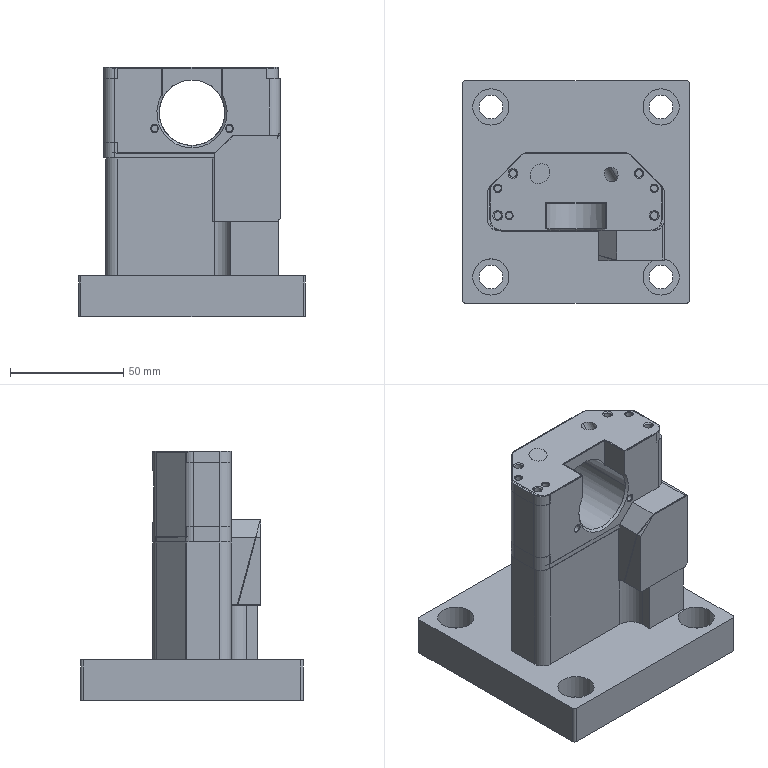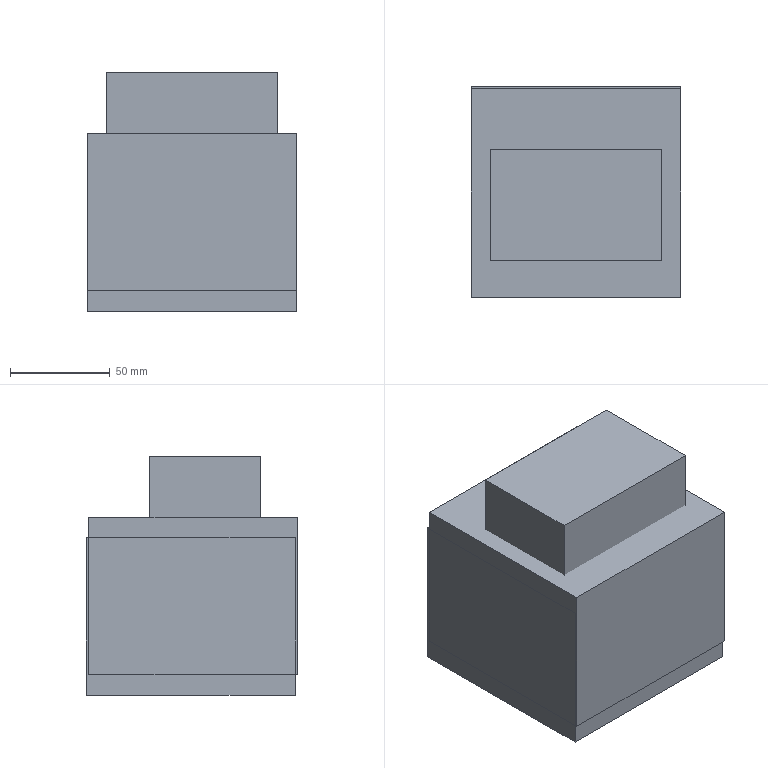CAM job | NX | 3-axis milling, 5-axis milling, drilling | part box 100 x 98 x 110 mm | stock box 104.975 x 105.953 x 119.645 mm
Tools:
number,name,description,diameter,corner_radius,flute_length,length,flutes
3,D4-12-D4-50-3T-ROUGH,D4-12-D4-50-3T-粗,4.0,0.0,12.0,50.0,2
9,D4-12-D4-50-3T-FINISH,D4-12-D4-50-3T,4.0,0.0,12.0,50.0,3
26,D6-18-D6-50-3T-ROUGH,D6-18-D6-50-3T-粗,6.0,0.0,18.0,50.0,2
8,D8-25-D8-60-3T-ROUGH,D8-25-D8-60-3T-粗,8.0,0.0,25.0,60.0,2
27,D8-25-D8-60-3T-FINISH,D8-25-D8-60-3T,8.0,0.0,25.0,60.0,3
0,D12-36-D12-75-3T-ROUGH,D12-36-D12-75-3T,12.0,0.0,36.0,75.0,3
0,D12-36-D12-120-3T-FINISH,D12-55-D12-120-3T,12.0,0.0,55.0,120.0,3
14,D16-48-D16-100-3T-FINISH,D16-48-D16-100-3T,16.0,0.0,48.0,100.0,3
2,D16-48-D16-100-3T-ROUGH,,16.0,0.0,45.0,100.0,2
0,D50面刀,D50面刀,50.0,0.0,30.0,30.0,4
1,D80面刀,D80面刀,80.0,0.0,30.0,30.0,5
4,点孔D6-65-90度,点孔D6-65-90度,6.0,0.0,0.0,65.0,2
15,点孔D8-79-90度,点孔D8-79-90度,8.0,0.0,0.0,79.0,2
8,钻头D2.8-39-67,钻刀D2.8-39-67,2.8,0.0,39.0,67.0,2
10,钻头D3.3-45-73,钻刀D3.3-45-73,3.3,0.0,45.0,73.0,2
9,钻头D4.2-54-83,钻刀D4.2-54-83,4.2,0.0,54.0,83.0,2
0,钻头D4.3-54-83,钻刀D4.3-54-83,4.3,0.0,54.0,83.0,2
4,钻头D5.1-62-92,钻刀D5.1-62-92,5.1,0.0,62.0,92.0,2
6,钻头D6.0-70-102,钻刀D6.0-70-102,6.0,0.0,70.0,102.0,2
7,钻头D6.5-73-105,钻刀D6.5-73-105,6.5,0.0,73.0,105.0,2
6,钻头D6.8-73-105,钻刀D6.8-73-105,6.8,0.0,73.0,105.0,2
5,钻头D8.0-81-114,钻刀D8.0-81-114,8.0,0.0,81.0,114.0,2
0,钻头D8.6-87-121,钻刀D8.6-87-121,8.6,0.0,87.0,121.0,2
5,上排M6-23-D6-63,上排M6-23-D6-63,6.0,0.0,23.0,26.0,2
0,上排M10-33-D7-74,上排M10-33-D7-74,10.0,0.0,33.0,38.0,2
0,倒角D6-90度,倒角D6-90度,6.0,0.0,5.0,50.0,2
3,倒角D8-90度,倒角D8-90度,8.0,0.0,8.0,60.0,2
0,倒角D12-90度,倒角D12-90度,12.0,0.0,10.0,75.0,2
11,D2.97插刀,Milling Tool-5 Parameters,2.97,0.0,50.0,75.0,2
12,螺纹铣刀M4-0.7,Thread Mill,3.16,0.0,10.0,50.0,2
16,D29镗刀,Milling Tool-5 Parameters,29.0,0.0,50.0,75.0,2
18,G1-2,Thread Mill,15.27,0.0,30.0,50.0,2
7,R1.75,Milling Tool-Ball Mill,3.5,1.75,50.0,75.0,2
30,T-2,Milling Tool-T Cutter,8.0,,1.5,25.0,4
29,D15.3,Drilling Tool,15.3,0.0,35.0,50.0,2
31,G4-1,Thread Mill,9.5,0.0,30.0,50.0,2
32,G3-8,Thread Mill,13.1,0.0,30.0,50.0,30
Operations:
program,operation,operation_type,tool,method,geometry_group,spindle_rpm,surface_speed,feed_per_tooth,feed_cut,feed_plunge,cut_length_mm,path_length_mm,cut_time_min,machine_time_min
A1,PLANAR_MILL,PlanarMilling,D80面刀,METHOD,A-G54,3500.0,879.0,0.0457,800.0,100.0,180.0,235.9,0.225,0.2306
A1,ADAPTIVE_MILLING,CavityMilling,D16-48-D16-100-3T-ROUGH,METHOD,WORKPIECE_54,6500.0,276.0,0.2273,2500.0,100.0,7545.599,7914.976,2.949,2.985
A1,FLOOR_WALL,VolumeBased25DMillingOperation,D12-36-D12-120-3T-FINISH,METHOD,WORKPIECE_54,4500.0,226.0,0.0889,800.0,100.0,222.319,276.319,0.2779,0.2833
A1,PLANAR_MILL_1,PlanarMilling,D12-36-D12-120-3T-FINISH,METHOD,WORKPIECE_54,4500.0,226.0,0.0889,800.0,100.0,369.078,479.078,0.4613,0.4723
A1,PLANAR_MILL_1_COPY,PlanarMilling,D12-36-D12-120-3T-FINISH,METHOD,WORKPIECE_54,4500.0,226.0,0.0889,800.0,100.0,106.138,218.138,0.1327,0.1439
A1,DRILLING,Operation,倒角D8-90度,METHOD,WORKPIECE_54,2000.0,50.0,0.05,200.0,0.0,6.1,72.2,0.0305,0.0371
A1,DRILLING_COPY,Operation,倒角D8-90度,METHOD,WORKPIECE_54,2000.0,50.0,0.05,200.0,0.0,6.1,128.2,0.0305,0.0427
A1,DRILLING_COPY_1,Operation,钻头D5.1-62-92,METHOD,WORKPIECE_54,2000.0,32.0,0.05,200.0,0.0,23.0,106.0,0.115,0.1233
A1,DRILLING_COPY_COPY,Operation,钻头D5.1-62-92,METHOD,WORKPIECE_54,2000.0,32.0,0.05,200.0,0.0,23.0,162.0,0.115,0.1289
A1,DRILLING_COPY_1_COPY,Operation,上排M6-23-D6-63,METHOD,WORKPIECE_54,400.0,7.0,0.5,400.0,0.0,18.0,96.0,0.045,0.0528
A1,DRILLING_COPY_COPY_COPY,Operation,上排M6-23-D6-63,METHOD,WORKPIECE_54,400.0,7.0,0.5,400.0,0.0,18.0,152.0,0.045,0.0584
B1,ADAPTIVE_MILLING_1,CavityMilling,D16-48-D16-100-3T-ROUGH,METHOD,WORKPIECE_55,6500.0,326.0,0.2308,3000.0,100.0,4872.012,4927.712,1.624,1.63
B1,ADAPTIVE_MILLING_1_COPY,CavityMilling,D16-48-D16-100-3T-ROUGH,METHOD,WORKPIECE_55,6500.0,326.0,0.2308,3000.0,100.0,6627.728,9490.539,1.798,2.084
B1,PLANAR_MILL_2,PlanarMilling,D16-48-D16-100-3T-ROUGH,METHOD,B-G55,5500.0,276.0,0.1091,1200.0,100.0,391.19,777.025,0.326,0.3646
B1,PLANAR_MILL_3,PlanarMilling,D16-48-D16-100-3T-ROUGH,METHOD,B-G55,5500.0,276.0,0.1091,1200.0,100.0,754.301,929.612,0.6286,0.6461
B1,PLANAR_MILL_4,PlanarMilling,D16-48-D16-100-3T-ROUGH,METHOD,B-G55,4500.0,226.0,0.1111,1000.0,100.0,388.921,424.921,0.3889,0.3925
B1,PLANAR_MILL_5,PlanarMilling,D16-48-D16-100-3T-ROUGH,METHOD,B-G55,5500.0,276.0,0.1091,1200.0,100.0,1491.555,1550.855,1.243,1.249
B1,PLANAR_MILL_5_COPY,PlanarMilling,D16-48-D16-100-3T-ROUGH,METHOD,B-G55,5500.0,276.0,0.1091,1200.0,100.0,214.664,302.364,0.1789,0.1877
B1,FLOOR_WALL_1_COPY,VolumeBased25DMillingOperation,D16-48-D16-100-3T-ROUGH,METHOD,B-G55,5500.0,276.0,0.1091,1200.0,100.0,423.865,491.832,0.3532,0.36
B1,PLANAR_MILL_6,PlanarMilling,D16-48-D16-100-3T-ROUGH,METHOD,B-G55,4500.0,226.0,0.1111,1000.0,100.0,175.054,291.055,0.1751,0.1867
B1,HOLE_MILLING,CylinderMilling,D4-12-D4-50-3T-ROUGH,METHOD,B-G55,4500.0,56.0,0.0889,800.0,100.0,96.442,137.442,0.1206,0.1247
B1,HOLE_MILLING_COPY,CylinderMilling,D4-12-D4-50-3T-ROUGH,METHOD,B-G55,4500.0,56.0,0.0889,800.0,100.0,48.54,90.54,0.0607,0.0649
B1,SPOT_DRILLING_1,HoleDrilling,点孔D6-65-90度,METHOD,B-G55,3000.0,56.0,0.0333,200.0,100.0,28.8,208.924,0.144,0.162
B1,SPOT_DRILLING,HoleDrilling,点孔D6-65-90度,METHOD,B-G55,3000.0,56.0,0.0333,200.0,100.0,40.0,271.14,0.2,0.2231
B1,SPOT_DRILLING_5,HoleDrilling,点孔D6-65-90度,METHOD,B-G55,3000.0,56.0,0.0333,200.0,100.0,10.0,44.0,0.05,0.0534
B1,SPOT_DRILLING_4,HoleDrilling,点孔D6-65-90度,METHOD,B-G55,3000.0,56.0,0.0333,200.0,100.0,13.0,47.0,0.065,0.0684
B1,SPOT_DRILLING_3,HoleDrilling,点孔D6-65-90度,METHOD,B-G55,3000.0,56.0,0.0333,200.0,100.0,19.2,120.2,0.096,0.1061
B1,SPOT_DRILLING_2,HoleDrilling,点孔D6-65-90度,METHOD,B-G55,3000.0,56.0,0.0333,200.0,100.0,23.2,126.2,0.116,0.1263
B1,SPOT_DRILLING_6,HoleDrilling,钻头D8.0-81-114,METHOD,B-G55,2000.0,50.0,0.05,200.0,100.0,264.0,298.0,1.32,1.323
B1,SPOT_DRILLING_7,HoleDrilling,钻头D6.0-70-102,METHOD,B-G55,2000.0,37.0,0.05,200.0,100.0,778.0,812.0,3.89,3.893
B1,SPOT_DRILLING_9,HoleDrilling,钻头D2.8-39-67,METHOD,B-G55,3000.0,31.0,0.0333,200.0,100.0,61.2,241.325,0.306,0.324
B1,SPOT_DRILLING_10,HoleDrilling,钻头D2.8-39-67,METHOD,B-G55,3000.0,31.0,0.0333,200.0,100.0,40.8,141.8,0.204,0.2141
B1,SPOT_DRILLING_11,HoleDrilling,钻头D4.2-54-83,METHOD,B-G55,3000.0,31.0,0.0333,200.0,100.0,41.2,144.2,0.206,0.2163
B1,SPOT_DRILLING_8,HoleDrilling,钻头D3.3-45-73,METHOD,B-G55,3000.0,31.0,0.0333,200.0,100.0,104.0,348.54,0.52,0.5445
B1,SPOT_DRILLING_9_COPY,HoleDrilling,D2.97插刀,METHOD,B-G55,3000.0,27.0,0.01,60.0,100.0,60.0,240.125,1.0,1.018
B1,SPOT_DRILLING_10_COPY,HoleDrilling,D2.97插刀,METHOD,B-G55,3000.0,27.0,0.01,60.0,100.0,40.0,141.0,0.6667,0.6768
B1,THREAD_MILLING,ThreadMilling,螺纹铣刀M4-0.7,METHOD,B-G55,4000.0,39.0,0.0125,100.0,100.0,402.713,938.053,4.027,4.081
B1,THREAD_MILLING_1,ThreadMilling,螺纹铣刀M4-0.7,METHOD,B-G55,4000.0,39.0,0.0125,100.0,100.0,366.046,609.302,3.66,3.685
B1,PLANAR_MILL_7,PlanarMilling,D16-48-D16-100-3T-FINISH,METHOD,B-G55,4500.0,226.0,0.0593,800.0,100.0,90.465,244.865,0.1131,0.1285
B1,PLANAR_MILL_6_COPY,PlanarMilling,D16-48-D16-100-3T-FINISH,METHOD,B-G55,4500.0,226.0,0.0593,800.0,100.0,353.637,670.327,0.442,0.4737
B1,PLANAR_MILL_6_COPY_COPY,PlanarMilling,D16-48-D16-100-3T-FINISH,METHOD,B-G55,4500.0,226.0,0.0593,800.0,100.0,101.196,312.429,0.1265,0.1476
B1,PLANAR_MILL_8,PlanarMilling,D16-48-D16-100-3T-FINISH,METHOD,B-G55,4500.0,226.0,0.0593,800.0,100.0,117.071,157.071,0.1463,0.1503
B1,PLANAR_MILL_8_COPY,PlanarMilling,D16-48-D16-100-3T-FINISH,METHOD,B-G55,4500.0,226.0,0.0593,800.0,100.0,117.699,157.679,0.1471,0.1511
B1,PLANAR_MILL_3_COPY,PlanarMilling,D16-48-D16-100-3T-FINISH,METHOD,B-G55,4500.0,226.0,0.0593,800.0,100.0,97.968,156.268,0.1225,0.1283
B1,PLANAR_MILL_12,PlanarMilling,D16-48-D16-100-3T-FINISH,METHOD,B-G55,4500.0,226.0,0.0593,800.0,100.0,74.555,205.355,0.0932,0.1063
B1,PLANAR_MILL_3_COPY_COPY,PlanarMilling,D16-48-D16-100-3T-FINISH,METHOD,B-G55,4500.0,226.0,0.0593,800.0,100.0,97.968,156.348,0.1225,0.1283
B1,PLANAR_MILL_2_COPY,PlanarMilling,D16-48-D16-100-3T-FINISH,METHOD,B-G55,4500.0,226.0,0.0593,800.0,100.0,111.562,155.642,0.1395,0.1439
B1,PLANAR_MILL_4_COPY,PlanarMilling,D16-48-D16-100-3T-FINISH,METHOD,B-G55,4500.0,226.0,0.0593,800.0,100.0,427.925,462.005,0.5349,0.5383
B1,PLANAR_MILL_22,PlanarMilling,D16-48-D16-100-3T-FINISH,METHOD,B-G55,5500.0,276.0,0.0364,600.0,100.0,176.451,401.7,0.2941,0.3166
B1,PLANAR_MILL_9,PlanarMilling,点孔D8-79-90度,METHOD,B-G55,3500.0,87.0,0.1429,1000.0,100.0,51.14,153.74,0.0511,0.0614
B1,PLANAR_MILL_9_COPY,PlanarMilling,点孔D8-79-90度,METHOD,B-G55,3500.0,87.0,0.1429,1000.0,100.0,66.801,106.801,0.0668,0.0708
B1,PLANAR_MILL_10,PlanarMilling,点孔D8-79-90度,METHOD,B-G55,3500.0,87.0,0.1429,1000.0,100.0,242.285,282.285,0.2423,0.2463
B1,PLANAR_MILL_10_COPY,PlanarMilling,点孔D8-79-90度,METHOD,B-G55,3500.0,87.0,0.1429,1000.0,100.0,141.876,180.876,0.1419,0.1458
B1,PLANAR_MILL_10_COPY_COPY,PlanarMilling,点孔D8-79-90度,METHOD,B-G55,3500.0,87.0,0.1429,1000.0,100.0,84.213,126.213,0.0842,0.0884
B1,CURVE_DRIVE,SurfaceContour,点孔D8-79-90度,METHOD,B-G55,4000.0,100.0,0.075,600.0,100.0,76.992,116.54,0.1283,0.1323
B1,PLANAR_MILL_21,PlanarMilling,D50面刀,METHOD,B-G55,4000.0,628.0,0.0375,600.0,100.0,141.942,178.042,0.2366,0.2402
B1,PLANAR_MILL_21_COPY,PlanarMilling,D50面刀,METHOD,B-G55,4000.0,628.0,0.0375,600.0,100.0,141.942,178.132,0.2366,0.2402
B1,3_AXIS_DEBURRING,TpMultiAxisDeburring,R1.75,METHOD,B-G55,4500.0,49.0,0.0667,600.0,90.0,206.897,290.896,0.3467,0.3467
B1,PLANAR_MILL_23,PlanarMilling,点孔D8-79-90度,METHOD,B-G55,4500.0,113.0,0.0889,800.0,100.0,20.529,57.529,0.0257,0.0294
B1,DRILLING_6,Operation,D29镗刀,METHOD,B-G55,1200.0,109.0,0.025,60.0,0.0,36.8,76.6,0.6133,0.6173
B1,DRILLING_6_COPY,Operation,D29镗刀,METHOD,B-G55,1200.0,109.0,0.025,60.0,0.0,36.8,76.6,0.6133,0.6173
C1,FLOOR_WALL_2_COPY,VolumeBased25DMillingOperation,D8-25-D8-60-3T-ROUGH,METHOD,C-G56,4500.0,113.0,0.1111,1000.0,100.0,203.324,263.324,0.2033,0.2093
C1,PLANAR_MILL_25_COPY,PlanarMilling,D8-25-D8-60-3T-ROUGH,METHOD,C-G56,6500.0,163.0,0.0923,1200.0,100.0,184.029,426.577,0.1534,0.1776
C1,PLANAR_MILL_25_COPY_COPY,PlanarMilling,D8-25-D8-60-3T-ROUGH,METHOD,C-G56,6500.0,163.0,0.0923,1200.0,100.0,184.029,420.577,0.1534,0.177
C1,FLOOR_WALL_1,VolumeBased25DMillingOperation,D8-25-D8-60-3T-ROUGH,METHOD,C-G56,6500.0,122.0,0.1154,1500.0,100.0,985.453,1362.547,0.657,0.6947
C1,FLOOR_WALL_1_COPY_3,VolumeBased25DMillingOperation,D8-25-D8-60-3T-ROUGH,METHOD,C-G56,6500.0,122.0,0.1154,1500.0,100.0,204.391,568.185,0.1363,0.1726
C1,PLANAR_MILL_24,PlanarMilling,D8-25-D8-60-3T-ROUGH,METHOD,C-G56,6500.0,122.0,0.1154,1500.0,100.0,70.0,124.0,0.0467,0.0521
C1,PLANAR_MILL_11,PlanarMilling,D8-25-D8-60-3T-ROUGH,METHOD,C-G56,6500.0,163.0,0.1154,1500.0,100.0,487.567,552.567,0.325,0.3315
C1,PLANAR_MILL_35,PlanarMilling,D8-25-D8-60-3T-ROUGH,METHOD,C-G56,4500.0,113.0,0.0593,800.0,100.0,39.106,104.906,0.0489,0.0555
C1,FLOOR_WALL_1_COPY_1_1,VolumeBased25DMillingOperation,D8-25-D8-60-3T-ROUGH,METHOD,C-G56,5500.0,172.0,0.1091,1200.0,100.0,1160.233,1396.07,0.9669,0.9904
C1,PLANAR_MILL_11_1,PlanarMilling,D8-25-D8-60-3T-ROUGH,METHOD,C-G56,5500.0,172.0,0.1091,1200.0,100.0,1353.427,1433.427,1.128,1.136
C1,PLANAR_MILL_11_1_COPY,PlanarMilling,D8-25-D8-60-3T-ROUGH,METHOD,C-G56,5500.0,172.0,0.1091,1200.0,100.0,194.887,254.887,0.1624,0.1684
C1,FLOOR_WALL_2,VolumeBased25DMillingOperation,D8-25-D8-60-3T-FINISH,METHOD,C-G56,4500.0,113.0,0.0593,800.0,100.0,203.324,263.324,0.2542,0.2602
C1,PLANAR_MILL_24_COPY,PlanarMilling,D8-25-D8-60-3T-FINISH,METHOD,C-G56,4500.0,113.0,0.0593,800.0,100.0,70.0,124.0,0.0875,0.0929
C1,FLOOR_WALL_1_COPY_2,VolumeBased25DMillingOperation,D8-25-D8-60-3T-FINISH,METHOD,C-G56,4500.0,113.0,0.0593,800.0,100.0,327.516,643.884,0.4094,0.441
C1,PLANAR_MILL_25,PlanarMilling,D8-25-D8-60-3T-FINISH,METHOD,C-G56,4500.0,113.0,0.0593,800.0,100.0,367.115,915.125,0.4589,0.5137
C1,PLANAR_MILL_25_COPY_2,PlanarMilling,D8-25-D8-60-3T-FINISH,METHOD,C-G56,4500.0,113.0,0.0593,800.0,100.0,94.971,334.445,0.1187,0.1427
C1,PLANAR_MILL_25_COPY_1,PlanarMilling,D8-25-D8-60-3T-FINISH,METHOD,C-G56,4500.0,113.0,0.0593,800.0,100.0,169.219,341.203,0.2115,0.2287
C1,FLOOR_WALL_1_COPY_3_COPY,VolumeBased25DMillingOperation,D8-25-D8-60-3T-FINISH,METHOD,C-G56,4500.0,113.0,0.0593,800.0,100.0,68.197,180.397,0.0852,0.0965
C1,PLANAR_MILL_35_COPY,PlanarMilling,D8-25-D8-60-3T-FINISH,METHOD,C-G56,4500.0,113.0,0.0593,800.0,100.0,38.949,104.949,0.0487,0.0553
C1,FLOOR_WALL_1_COPY_1_1_COPY,VolumeBased25DMillingOperation,D8-25-D8-60-3T-FINISH,METHOD,C-G56,4500.0,113.0,0.0593,800.0,100.0,290.058,356.058,0.3626,0.3692
C1,DRILLING_7,Operation,点孔D6-65-90度,METHOD,C-G56,2500.0,47.0,0.04,200.0,0.0,15.0,79.189,0.075,0.0814
C1,DRILLING_1_COPY,Operation,D6-18-D6-50-3T-ROUGH,METHOD,C-G56,1600.0,30.0,0.0469,150.0,0.0,25.6,54.2,0.1707,0.1735
C1,SPOT_DRILLING_14,HoleDrilling,钻头D3.3-45-73,METHOD,C-G56,3000.0,31.0,0.0333,200.0,100.0,48.0,170.0,0.24,0.2522
C1,DRILLING_9,Operation,D15.3,METHOD,C-G56,1600.0,30.0,0.0469,150.0,0.0,29.797,62.593,0.1986,0.2019
C1,PLANAR_MILL_37,PlanarMilling,D8-25-D8-60-3T-ROUGH,METHOD,C-G56,4500.0,113.0,0.1111,1000.0,100.0,296.726,365.526,0.2967,0.3036
C1,PLANAR_MILL_26_COPY_1,PlanarMilling,T-2,METHOD,C-G56,3000.0,75.0,0.0417,500.0,100.0,28.16,89.96,0.0563,0.0625
C1,PLANAR_MILL_26_COPY_COPY,PlanarMilling,T-2,METHOD,C-G56,3000.0,75.0,0.0417,500.0,100.0,30.102,89.102,0.0602,0.0661
C1,PLANAR_MILL_26,PlanarMilling,T-2,METHOD,C-G56,3000.0,75.0,0.0417,500.0,100.0,30.767,92.767,0.0615,0.0677
C1,PLANAR_MILL_26_COPY,PlanarMilling,T-2,METHOD,C-G56,3000.0,75.0,0.0417,500.0,100.0,30.767,89.767,0.0615,0.0674
C1,PLANAR_MILL_27,PlanarMilling,点孔D8-79-90度,METHOD,C-G56,3500.0,87.0,0.1429,1000.0,100.0,117.774,177.774,0.1178,0.1238
C1,PLANAR_MILL_27_COPY,PlanarMilling,点孔D8-79-90度,METHOD,C-G56,3500.0,87.0,0.1429,1000.0,100.0,36.505,98.505,0.0365,0.0427
C1,PLANAR_MILL_27_COPY_COPY,PlanarMilling,点孔D8-79-90度,METHOD,C-G56,3500.0,87.0,0.1429,1000.0,100.0,49.802,110.802,0.0498,0.0559
C1,PLANAR_MILL_28,PlanarMilling,点孔D8-79-90度,METHOD,C-G56,3500.0,87.0,0.1429,1000.0,100.0,118.607,331.245,0.1186,0.1399
C1,PLANAR_MILL_28_COPY_1,PlanarMilling,点孔D8-79-90度,METHOD,C-G56,3500.0,87.0,0.1429,1000.0,100.0,21.812,114.812,0.0218,0.0311
C1,PLANAR_MILL_28_COPY,PlanarMilling,点孔D8-79-90度,METHOD,C-G56,3500.0,87.0,0.1429,1000.0,100.0,76.106,228.24,0.0761,0.0913
C1,PLANAR_MILL_28_COPY_COPY,PlanarMilling,点孔D8-79-90度,METHOD,C-G56,3500.0,87.0,0.1429,1000.0,100.0,45.883,166.383,0.0459,0.0579
C1,PLANAR_MILL_9_COPY_COPY_COPY,PlanarMilling,点孔D8-79-90度,METHOD,C-G56,3500.0,87.0,0.1429,1000.0,100.0,63.085,124.085,0.0631,0.0692
C1,PLANAR_MILL_9_COPY_COPY,PlanarMilling,点孔D8-79-90度,METHOD,C-G56,3500.0,87.0,0.1429,1000.0,100.0,51.035,111.034,0.051,0.057
C1,PLANAR_MILL_9_COPY_COPY_COPY_1,PlanarMilling,点孔D8-79-90度,METHOD,C-G56,3500.0,87.0,0.1429,1000.0,100.0,55.53,115.53,0.0555,0.0615
C1,PLANAR_MILL_9_COPY_COPY_COPY_1_COPY,PlanarMilling,点孔D8-79-90度,METHOD,C-G56,3500.0,87.0,0.1429,1000.0,100.0,31.99,91.99,0.032,0.038
C1,THREAD_MILLING_2_1,ThreadMilling,G1-2,METHOD,C-G56,4500.0,221.0,0.0222,200.0,100.0,142.231,251.869,0.7112,0.7221
C1,THREAD_MILLING_3,ThreadMilling,G4-1,METHOD,C-G56,4500.0,221.0,0.0222,200.0,100.0,88.577,180.193,0.4429,0.452
C1,THREAD_MILLING_4,ThreadMilling,G3-8,METHOD,C-G56,4500.0,221.0,0.0222,200.0,100.0,109.302,219.032,0.5465,0.5575
C1,THREAD_MILLING_5,ThreadMilling,螺纹铣刀M4-0.7,METHOD,C-G56,4500.0,44.0,0.0222,200.0,100.0,236.123,439.594,1.181,1.201
工装1,FLOOR_WALL_3,VolumeBased25DMillingOperation,D80面刀,METHOD,GZ1,3500.0,879.0,0.0457,800.0,100.0,418.002,452.002,0.5225,0.5259
工装1,ADAPTIVE_MILLING_2,CavityMilling,D16-48-D16-100-3T-ROUGH,METHOD,WORKPIECE,5500.0,276.0,0.2273,2500.0,100.0,1739.726,1833.165,0.6959,0.7052
工装1,PLANAR_MILL_13,PlanarMilling,D12-36-D12-75-3T-ROUGH,METHOD,GZ1,4500.0,169.0,0.0593,800.0,100.0,444.327,540.188,0.5554,0.565
工装1,DRILLING_2,Operation,倒角D8-90度,METHOD,GZ1,2000.0,50.0,0.05,200.0,0.0,36.0,440.855,0.18,0.2205
工装1,DRILLING_3,Operation,钻头D6.8-73-105,METHOD,GZ1,2000.0,42.0,0.05,200.0,0.0,92.0,458.216,0.46,0.4966
工装1,DRILLING_4,Operation,钻头D6.8-73-105,METHOD,GZ1,2000.0,42.0,0.05,200.0,0.0,26.0,175.06,0.13,0.1449
工装1,DRILLING_5,Operation,钻头D6.5-73-105,METHOD,GZ1,2500.0,51.0,0.04,200.0,0.0,53.0,146,0.265,0.2743
工装1,DRILLING_5_COPY,Operation,钻头D6.5-73-105,METHOD,GZ1,2500.0,51.0,0.04,200.0,0.0,75.0,190,0.375,0.3865
工装1,PLANAR_MILL_14,PlanarMilling,D8-25-D8-60-3T-ROUGH,METHOD,GZ1,4500.0,113.0,0.1111,1000.0,100.0,2333.795,2514.209,2.334,2.352
工装1,PLANAR_MILL_15_COPY,PlanarMilling,D4-12-D4-50-3T-FINISH,METHOD,GZ1,4500.0,56.0,0.0741,1000.0,100.0,455.61,634.784,0.4556,0.4735
工装1,PLANAR_MILL_15,PlanarMilling,D4-12-D4-50-3T-FINISH,METHOD,GZ1,4500.0,56.0,0.0444,600.0,100.0,72.806,265.666,0.1213,0.1406
工装1,PLANAR_MILL_19,PlanarMilling,D4-12-D4-50-3T-FINISH,METHOD,GZ1,4500.0,56.0,0.0741,1000.0,100.0,930.074,1340.125,0.9301,0.9711
工装1,PLANAR_MILL_16,PlanarMilling,倒角D8-90度,METHOD,GZ1,3500.0,87.0,0.1143,800.0,100.0,110.096,577.645,0.1376,0.1844
工装1,PLANAR_MILL_16_COPY,PlanarMilling,倒角D8-90度,METHOD,GZ1,3500.0,87.0,0.1143,800.0,100.0,426.624,465.627,0.5333,0.5372
工装2,ADAPTIVE_MILLING_3,CavityMilling,D16-48-D16-100-3T-ROUGH,METHOD,WORKPIECE_1,6500.0,326.0,0.1923,2500.0,100.0,31700.91,32185.157,12.593,12.642
工装2,FLOOR_WALL_4,VolumeBased25DMillingOperation,D12-36-D12-75-3T-ROUGH,METHOD,GZ2,5500.0,207.0,0.0485,800.0,100.0,309.617,363.617,0.387,0.3924
工装2,FLOOR_WALL_4_COPY,VolumeBased25DMillingOperation,D12-36-D12-75-3T-ROUGH,METHOD,GZ2,5500.0,207.0,0.0485,800.0,100.0,179.958,289.958,0.2249,0.2359
工装2,PLANAR_MILL_17,PlanarMilling,D12-36-D12-75-3T-ROUGH,METHOD,GZ2,5500.0,207.0,0.0485,800.0,100.0,62.55,174.412,0.0782,0.0894
工装2,PLANAR_MILL_18,PlanarMilling,D8-25-D8-60-3T-ROUGH,METHOD,GZ2,4500.0,113.0,0.0889,800.0,100.0,2854.687,3780.122,3.568,3.661
工装3,SPOT_DRILLING_13,HoleDrilling,倒角D12-90度,METHOD,GZ3,2000.0,75.0,0.05,200.0,100.0,54.0,520.659,0.27,0.3167
工装3,SPOT_DRILLING_13_COPY,HoleDrilling,钻头D8.6-87-121,METHOD,GZ3,2000.0,75.0,0.05,200.0,100.0,264.0,625.0,1.32,1.356
工装3,PLANAR_MILL_20,PlanarMilling,D4-12-D4-50-3T-ROUGH,METHOD,GZ3,4500.0,56.0,0.0667,600.0,100.0,1403.673,1578.955,2.34,2.357
工装3,SPOT_DRILLING_13_COPY_1,HoleDrilling,倒角D12-90度,METHOD,GZ3,2000.0,75.0,0.05,200.0,100.0,96.0,562.659,0.48,0.5267
工装3,SPOT_DRILLING_13_COPY_COPY,HoleDrilling,上排M10-33-D7-74,METHOD,GZ3,300.0,9.0,0.75,450.0,100.0,64.0,425.0,0.1422,0.1783
工装3,PLANAR_MILL_20_COPY,PlanarMilling,D4-12-D4-50-3T-ROUGH,METHOD,GZ3,4500.0,56.0,0.0667,600.0,100.0,42.505,234.506,0.0708,0.09
工装4,PLANAR_MILL_29,PlanarMilling,D80面刀,METHOD,GZ4,3500.0,879.0,0.0571,1000.0,100.0,532.0,865.962,0.532,0.5654
工装4,PLANAR_MILL_30,PlanarMilling,D16-48-D16-100-3T-ROUGH,METHOD,GZ4,4500.0,226.0,0.1667,1500.0,100.0,7008.451,8152.451,4.672,4.787
工装4,PLANAR_MILL_30_COPY,PlanarMilling,D16-48-D16-100-3T-ROUGH,METHOD,GZ4,4500.0,226.0,0.0741,1000.0,100.0,916.386,1107.564,0.9164,0.9355
工装4,DRILLING_10,Operation,倒角D8-90度,METHOD,GZ4,2000.0,50.0,0.05,200.0,0.0,45.0,487.622,0.225,0.2693
工装4,DRILLING_10_COPY,Operation,钻头D6.8-73-105,METHOD,GZ4,2000.0,50.0,0.05,200.0,0.0,230.0,773.242,1.15,1.204
工装4,PLANAR_MILL_31,PlanarMilling,D4-12-D4-50-3T-ROUGH,METHOD,GZ4,4000.0,50.0,0.125,1000.0,100.0,1465.059,1877.549,1.465,1.506
工装4,PLANAR_MILL_31_COPY,PlanarMilling,D4-12-D4-50-3T-ROUGH,METHOD,GZ4,4000.0,50.0,0.125,1000.0,100.0,303.245,471.921,0.3032,0.3201
工装4,PLANAR_MILL_31_COPY_COPY,PlanarMilling,D4-12-D4-50-3T-ROUGH,METHOD,GZ4,4000.0,50.0,0.075,600.0,100.0,75.954,267.967,0.1266,0.1458
工装4,DRILLING_11,Operation,D8-25-D8-60-3T-ROUGH,METHOD,GZ4,2000.0,50.0,0.0375,150.0,0.0,92.0,342.058,0.6133,0.6383
工装4,PLANAR_MILL_32,PlanarMilling,倒角D6-90度,METHOD,GZ4,3000.0,56.0,0.1667,1000.0,100.0,415.708,454.708,0.4157,0.4196
工装4,PLANAR_MILL_32_COPY,PlanarMilling,倒角D6-90度,METHOD,GZ4,3000.0,56.0,0.1667,1000.0,100.0,269.416,933.403,0.2694,0.3358
工装5,PLANAR_MILL_33,PlanarMilling,D8-25-D8-60-3T-ROUGH,METHOD,GZ5,4500.0,113.0,0.1111,1000.0,100.0,5415.426,5937.523,5.415,5.468
工装5,PLANAR_MILL_34,PlanarMilling,倒角D6-90度,METHOD,GZ5,3500.0,65.0,0.1429,1000.0,100.0,413.35,472.35,0.4134,0.4193
工装5,PLANAR_MILL_34_COPY,PlanarMilling,倒角D6-90度,METHOD,GZ5,3500.0,65.0,0.1429,1000.0,100.0,236.94,712.508,0.2369,0.2845
工装5,FLOOR_WALL_5,VolumeBased25DMillingOperation,D4-12-D4-50-3T-ROUGH,METHOD,GZ5,5500.0,69.0,0.0909,1000.0,100.0,7024.099,7647.088,7.024,7.086
工装5,FLOOR_WALL_5_COPY,VolumeBased25DMillingOperation,D4-12-D4-50-3T-ROUGH,METHOD,GZ5,4500.0,56.0,0.0889,800.0,100.0,868.697,932.697,1.086,1.092
工装5,DRILLING_12,Operation,点孔D6-65-90度,METHOD,GZ5,2000.0,37.0,0.05,200.0,0.0,20.8,263.342,0.104,0.1283
工装5,PLANAR_MILL_36,PlanarMilling,点孔D6-65-90度,METHOD,GZ5,3500.0,65.0,0.1429,1000.0,100.0,209.552,268.551,0.2096,0.2155
工装5,DRILLING_12_COPY,Operation,钻头D4.3-54-83,METHOD,GZ5,2000.0,27.0,0.05,200.0,0.0,44.0,309.742,0.22,0.2466
工装5,FLOOR_WALL_5_COPY_COPY,VolumeBased25DMillingOperation,D4-12-D4-50-3T-ROUGH,METHOD,GZ5,4500.0,56.0,0.0889,800.0,100.0,209.451,273.451,0.2618,0.2682